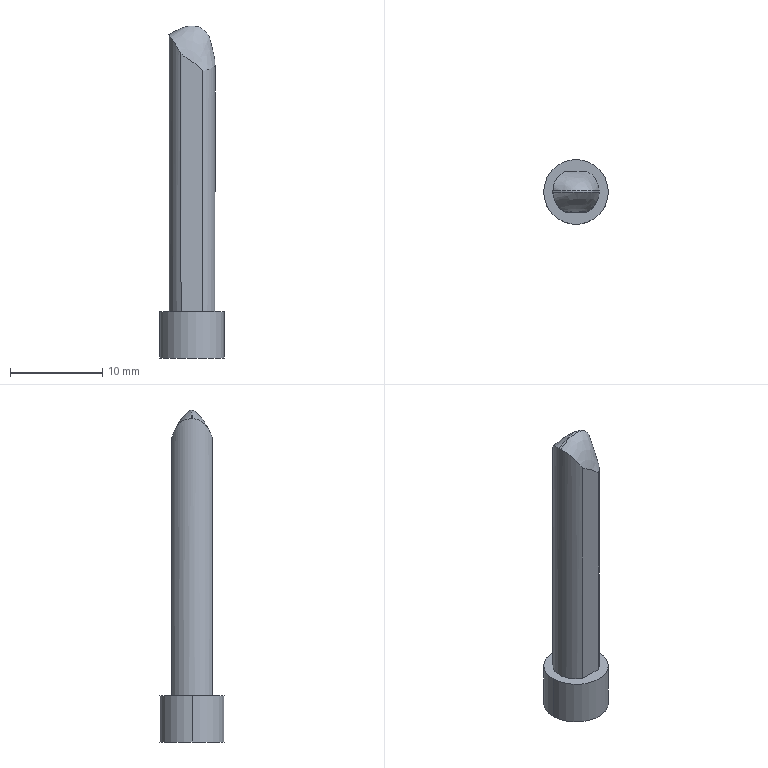Part | 1 solid | 14 faces | box 7 x 7 x 35.941 mm | volume 740.392 mm3 | plane 5 | cylinder 5 | spline 4 | commonest cylinder face diameters 5 x2 7 x2 3.9 x1